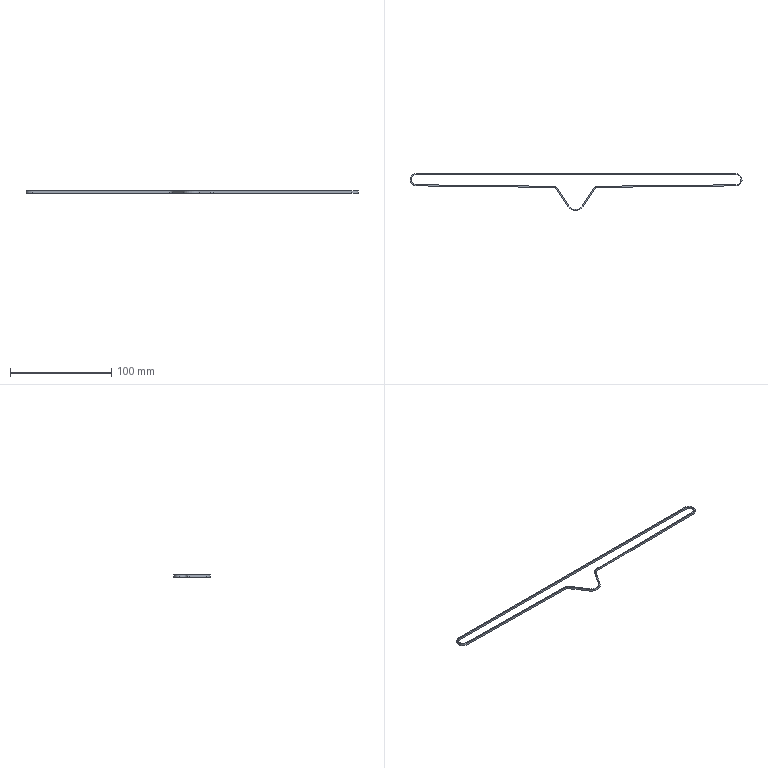Part | NX | features BREP 1 | 1 solid | 24 faces | box 328.22 x 36.55 x 2 mm | volume 1530 mm3 | plane 12 | cylinder 12 | commonest cylinder face diameters 10 x5 12.22 x3 7.78 x2 15.66 x1 17.88 x1
STEP:
#1=CARTESIAN_POINT('',(-136.555,-6.5,-1.));
#2=VERTEX_POINT('',#1);
#3=CARTESIAN_POINT('',(0.05492,-5.,-1.));
#4=VERTEX_POINT('',#3);
#5=CARTESIAN_POINT('',(0.05492,-5.,-1.));
#6=DIRECTION('',(0.9999,0.01098,0.));
#7=VECTOR('',#6,1000.);
#8=LINE('',#5,#7);
#9=EDGE_CURVE('',#2,#4,#8,.T.);
#10=ORIENTED_EDGE('',*,*,#9,.F.);
#11=CARTESIAN_POINT('',(-136.555,-6.5,1.));
#12=VERTEX_POINT('',#11);
#13=CARTESIAN_POINT('',(-136.555,-6.5,1.));
#14=DIRECTION('',(0.,0.,-1.));
#15=VECTOR('',#14,1000.);
#16=LINE('',#13,#15);
#17=EDGE_CURVE('',#12,#2,#16,.T.);
#18=ORIENTED_EDGE('',*,*,#17,.F.);
#19=CARTESIAN_POINT('',(0.05492,-5.,1.));
#20=VERTEX_POINT('',#19);
#21=CARTESIAN_POINT('',(0.05492,-5.,1.));
#22=DIRECTION('',(0.9999,0.01098,0.));
#23=VECTOR('',#22,1000.);
#24=LINE('',#21,#23);
#25=EDGE_CURVE('',#12,#20,#24,.T.);
#26=ORIENTED_EDGE('',*,*,#25,.T.);
#27=CARTESIAN_POINT('',(0.05492,-5.,1.));
#28=DIRECTION('',(0.,0.,-1.));
#29=VECTOR('',#28,1000.);
#30=LINE('',#27,#29);
#31=EDGE_CURVE('',#20,#4,#30,.T.);
#32=ORIENTED_EDGE('',*,*,#31,.T.);
#33=EDGE_LOOP('',(#10,#18,#26,#32));
#34=FACE_BOUND('',#33,.T.);
#35=CARTESIAN_POINT('',(0.05492,-5.,1.));
#36=DIRECTION('',(-0.01098,0.9999,0.));
#37=DIRECTION('',(-0.9999,-0.01098,0.));
#38=AXIS2_PLACEMENT_3D('',#35,#36,#37);
#39=PLANE('',#38);
#40=ADVANCED_FACE('',(#34),#39,.T.);
#41=CARTESIAN_POINT('',(-140.67,-8.741,-1.));
#42=VERTEX_POINT('',#41);
#43=CARTESIAN_POINT('',(-136.5,-11.5,-1.));
#44=DIRECTION('',(0.,0.,-1.));
#45=DIRECTION('',(1.,0.,0.));
#46=AXIS2_PLACEMENT_3D('',#43,#44,#45);
#47=CIRCLE('',#46,5.);
#48=EDGE_CURVE('',#42,#2,#47,.T.);
#49=ORIENTED_EDGE('',*,*,#48,.F.);
#50=CARTESIAN_POINT('',(-140.67,-8.741,1.));
#51=VERTEX_POINT('',#50);
#52=CARTESIAN_POINT('',(-140.67,-8.741,1.));
#53=DIRECTION('',(0.,0.,-1.));
#54=VECTOR('',#53,1000.);
#55=LINE('',#52,#54);
#56=EDGE_CURVE('',#51,#42,#55,.T.);
#57=ORIENTED_EDGE('',*,*,#56,.F.);
#58=CARTESIAN_POINT('',(-136.5,-11.5,1.));
#59=DIRECTION('',(0.,0.,-1.));
#60=DIRECTION('',(1.,0.,0.));
#61=AXIS2_PLACEMENT_3D('',#58,#59,#60);
#62=CIRCLE('',#61,5.);
#63=EDGE_CURVE('',#51,#12,#62,.T.);
#64=ORIENTED_EDGE('',*,*,#63,.T.);
#65=ORIENTED_EDGE('',*,*,#17,.T.);
#66=EDGE_LOOP('',(#49,#57,#64,#65));
#67=FACE_BOUND('',#66,.T.);
#68=CARTESIAN_POINT('',(-136.5,-11.5,1.));
#69=DIRECTION('',(0.,0.,-1.));
#70=DIRECTION('',(-1.,0.,0.));
#71=AXIS2_PLACEMENT_3D('',#68,#69,#70);
#72=CYLINDRICAL_SURFACE('',#71,5.);
#73=ADVANCED_FACE('',(#67),#72,.T.);
#74=CARTESIAN_POINT('',(-151.97,-25.82,-1.));
#75=VERTEX_POINT('',#74);
#76=CARTESIAN_POINT('',(-140.67,-8.741,-1.));
#77=DIRECTION('',(0.5518,0.834,0.));
#78=VECTOR('',#77,1000.);
#79=LINE('',#76,#78);
#80=EDGE_CURVE('',#75,#42,#79,.T.);
#81=ORIENTED_EDGE('',*,*,#80,.F.);
#82=CARTESIAN_POINT('',(-151.97,-25.82,1.));
#83=VERTEX_POINT('',#82);
#84=CARTESIAN_POINT('',(-151.97,-25.82,1.));
#85=DIRECTION('',(0.,0.,-1.));
#86=VECTOR('',#85,1000.);
#87=LINE('',#84,#86);
#88=EDGE_CURVE('',#83,#75,#87,.T.);
#89=ORIENTED_EDGE('',*,*,#88,.F.);
#90=CARTESIAN_POINT('',(-140.67,-8.741,1.));
#91=DIRECTION('',(0.5518,0.834,0.));
#92=VECTOR('',#91,1000.);
#93=LINE('',#90,#92);
#94=EDGE_CURVE('',#83,#51,#93,.T.);
#95=ORIENTED_EDGE('',*,*,#94,.T.);
#96=ORIENTED_EDGE('',*,*,#56,.T.);
#97=EDGE_LOOP('',(#81,#89,#95,#96));
#98=FACE_BOUND('',#97,.T.);
#99=CARTESIAN_POINT('',(-140.67,-8.741,1.));
#100=DIRECTION('',(-0.834,0.5518,0.));
#101=DIRECTION('',(-0.5518,-0.834,0.));
#102=AXIS2_PLACEMENT_3D('',#99,#100,#101);
#103=PLANE('',#102);
#104=ADVANCED_FACE('',(#98),#103,.T.);
#105=CARTESIAN_POINT('',(-165.03,-25.82,-1.));
#106=VERTEX_POINT('',#105);
#107=CARTESIAN_POINT('',(-158.5,-21.5,-1.));
#108=DIRECTION('',(0.,0.,1.));
#109=DIRECTION('',(-1.,0.,0.));
#110=AXIS2_PLACEMENT_3D('',#107,#108,#109);
#111=CIRCLE('',#110,7.83);
#112=EDGE_CURVE('',#106,#75,#111,.T.);
#113=ORIENTED_EDGE('',*,*,#112,.F.);
#114=CARTESIAN_POINT('',(-165.03,-25.82,1.));
#115=VERTEX_POINT('',#114);
#116=CARTESIAN_POINT('',(-165.03,-25.82,1.));
#117=DIRECTION('',(0.,0.,-1.));
#118=VECTOR('',#117,1000.);
#119=LINE('',#116,#118);
#120=EDGE_CURVE('',#115,#106,#119,.T.);
#121=ORIENTED_EDGE('',*,*,#120,.F.);
#122=CARTESIAN_POINT('',(-158.5,-21.5,1.));
#123=DIRECTION('',(0.,0.,1.));
#124=DIRECTION('',(-1.,0.,0.));
#125=AXIS2_PLACEMENT_3D('',#122,#123,#124);
#126=CIRCLE('',#125,7.83);
#127=EDGE_CURVE('',#115,#83,#126,.T.);
#128=ORIENTED_EDGE('',*,*,#127,.T.);
#129=ORIENTED_EDGE('',*,*,#88,.T.);
#130=EDGE_LOOP('',(#113,#121,#128,#129));
#131=FACE_BOUND('',#130,.T.);
#132=CARTESIAN_POINT('',(-158.5,-21.5,1.));
#133=DIRECTION('',(0.,0.,-1.));
#134=DIRECTION('',(-1.,0.,0.));
#135=AXIS2_PLACEMENT_3D('',#132,#133,#134);
#136=CYLINDRICAL_SURFACE('',#135,7.83);
#137=ADVANCED_FACE('',(#131),#136,.F.);
#138=CARTESIAN_POINT('',(-176.33,-8.741,-1.));
#139=VERTEX_POINT('',#138);
#140=CARTESIAN_POINT('',(-165.03,-25.82,-1.));
#141=DIRECTION('',(0.5518,-0.834,0.));
#142=VECTOR('',#141,1000.);
#143=LINE('',#140,#142);
#144=EDGE_CURVE('',#139,#106,#143,.T.);
#145=ORIENTED_EDGE('',*,*,#144,.F.);
#146=CARTESIAN_POINT('',(-176.33,-8.741,1.));
#147=VERTEX_POINT('',#146);
#148=CARTESIAN_POINT('',(-176.33,-8.741,1.));
#149=DIRECTION('',(0.,0.,-1.));
#150=VECTOR('',#149,1000.);
#151=LINE('',#148,#150);
#152=EDGE_CURVE('',#147,#139,#151,.T.);
#153=ORIENTED_EDGE('',*,*,#152,.F.);
#154=CARTESIAN_POINT('',(-165.03,-25.82,1.));
#155=DIRECTION('',(0.5518,-0.834,0.));
#156=VECTOR('',#155,1000.);
#157=LINE('',#154,#156);
#158=EDGE_CURVE('',#147,#115,#157,.T.);
#159=ORIENTED_EDGE('',*,*,#158,.T.);
#160=ORIENTED_EDGE('',*,*,#120,.T.);
#161=EDGE_LOOP('',(#145,#153,#159,#160));
#162=FACE_BOUND('',#161,.T.);
#163=CARTESIAN_POINT('',(-165.03,-25.82,1.));
#164=DIRECTION('',(0.834,0.5518,0.));
#165=DIRECTION('',(-0.5518,0.834,0.));
#166=AXIS2_PLACEMENT_3D('',#163,#164,#165);
#167=PLANE('',#166);
#168=ADVANCED_FACE('',(#162),#167,.T.);
#169=CARTESIAN_POINT('',(-180.445,-6.5,-1.));
#170=VERTEX_POINT('',#169);
#171=CARTESIAN_POINT('',(-180.5,-11.5,-1.));
#172=DIRECTION('',(0.,0.,-1.));
#173=DIRECTION('',(1.,0.,0.));
#174=AXIS2_PLACEMENT_3D('',#171,#172,#173);
#175=CIRCLE('',#174,5.);
#176=EDGE_CURVE('',#170,#139,#175,.T.);
#177=ORIENTED_EDGE('',*,*,#176,.F.);
#178=CARTESIAN_POINT('',(-180.445,-6.5,1.));
#179=VERTEX_POINT('',#178);
#180=CARTESIAN_POINT('',(-180.445,-6.5,1.));
#181=DIRECTION('',(0.,0.,-1.));
#182=VECTOR('',#181,1000.);
#183=LINE('',#180,#182);
#184=EDGE_CURVE('',#179,#170,#183,.T.);
#185=ORIENTED_EDGE('',*,*,#184,.F.);
#186=CARTESIAN_POINT('',(-180.5,-11.5,1.));
#187=DIRECTION('',(0.,0.,-1.));
#188=DIRECTION('',(1.,0.,0.));
#189=AXIS2_PLACEMENT_3D('',#186,#187,#188);
#190=CIRCLE('',#189,5.);
#191=EDGE_CURVE('',#179,#147,#190,.T.);
#192=ORIENTED_EDGE('',*,*,#191,.T.);
#193=ORIENTED_EDGE('',*,*,#152,.T.);
#194=EDGE_LOOP('',(#177,#185,#192,#193));
#195=FACE_BOUND('',#194,.T.);
#196=CARTESIAN_POINT('',(-180.5,-11.5,1.));
#197=DIRECTION('',(0.,0.,-1.));
#198=DIRECTION('',(-1.,0.,0.));
#199=AXIS2_PLACEMENT_3D('',#196,#197,#198);
#200=CYLINDRICAL_SURFACE('',#199,5.);
#201=ADVANCED_FACE('',(#195),#200,.T.);
#202=CARTESIAN_POINT('',(-316.055,-5.,-1.));
#203=VERTEX_POINT('',#202);
#204=CARTESIAN_POINT('',(-180.445,-6.5,-1.));
#205=DIRECTION('',(0.9999,-0.01106,0.));
#206=VECTOR('',#205,1000.);
#207=LINE('',#204,#206);
#208=EDGE_CURVE('',#203,#170,#207,.T.);
#209=ORIENTED_EDGE('',*,*,#208,.F.);
#210=CARTESIAN_POINT('',(-316.055,-5.,1.));
#211=VERTEX_POINT('',#210);
#212=CARTESIAN_POINT('',(-316.055,-5.,1.));
#213=DIRECTION('',(0.,0.,-1.));
#214=VECTOR('',#213,1000.);
#215=LINE('',#212,#214);
#216=EDGE_CURVE('',#211,#203,#215,.T.);
#217=ORIENTED_EDGE('',*,*,#216,.F.);
#218=CARTESIAN_POINT('',(-180.445,-6.5,1.));
#219=DIRECTION('',(0.9999,-0.01106,0.));
#220=VECTOR('',#219,1000.);
#221=LINE('',#218,#220);
#222=EDGE_CURVE('',#211,#179,#221,.T.);
#223=ORIENTED_EDGE('',*,*,#222,.T.);
#224=ORIENTED_EDGE('',*,*,#184,.T.);
#225=EDGE_LOOP('',(#209,#217,#223,#224));
#226=FACE_BOUND('',#225,.T.);
#227=CARTESIAN_POINT('',(-180.445,-6.5,1.));
#228=DIRECTION('',(0.01106,0.9999,0.));
#229=DIRECTION('',(-0.9999,0.01106,0.));
#230=AXIS2_PLACEMENT_3D('',#227,#228,#229);
#231=PLANE('',#230);
#232=ADVANCED_FACE('',(#226),#231,.T.);
#233=CARTESIAN_POINT('',(-321.,0.,1.));
#234=VERTEX_POINT('',#233);
#235=CARTESIAN_POINT('',(-321.,0.,-1.));
#236=VERTEX_POINT('',#235);
#237=CARTESIAN_POINT('',(-321.,0.,1.));
#238=DIRECTION('',(0.,0.,-1.));
#239=VECTOR('',#238,1000.);
#240=LINE('',#237,#239);
#241=EDGE_CURVE('',#234,#236,#240,.T.);
#242=ORIENTED_EDGE('',*,*,#241,.F.);
#243=CARTESIAN_POINT('',(-316.,0.,1.));
#244=DIRECTION('',(0.,0.,1.));
#245=DIRECTION('',(-1.,0.,0.));
#246=AXIS2_PLACEMENT_3D('',#243,#244,#245);
#247=CIRCLE('',#246,5.);
#248=EDGE_CURVE('',#234,#211,#247,.T.);
#249=ORIENTED_EDGE('',*,*,#248,.T.);
#250=ORIENTED_EDGE('',*,*,#216,.T.);
#251=CARTESIAN_POINT('',(-316.,0.,-1.));
#252=DIRECTION('',(0.,0.,1.));
#253=DIRECTION('',(-1.,0.,0.));
#254=AXIS2_PLACEMENT_3D('',#251,#252,#253);
#255=CIRCLE('',#254,5.);
#256=EDGE_CURVE('',#236,#203,#255,.T.);
#257=ORIENTED_EDGE('',*,*,#256,.F.);
#258=EDGE_LOOP('',(#242,#249,#250,#257));
#259=FACE_BOUND('',#258,.T.);
#260=CARTESIAN_POINT('',(-316.,0.,1.));
#261=DIRECTION('',(0.,0.,-1.));
#262=DIRECTION('',(-1.,0.,0.));
#263=AXIS2_PLACEMENT_3D('',#260,#261,#262);
#264=CYLINDRICAL_SURFACE('',#263,5.);
#265=ADVANCED_FACE('',(#259),#264,.F.);
#266=CARTESIAN_POINT('',(0.,5.,-1.));
#267=VERTEX_POINT('',#266);
#268=CARTESIAN_POINT('',(-316.,5.,-1.));
#269=VERTEX_POINT('',#268);
#270=CARTESIAN_POINT('',(-316.,5.,-1.));
#271=DIRECTION('',(-1.,0.,0.));
#272=VECTOR('',#271,1000.);
#273=LINE('',#270,#272);
#274=EDGE_CURVE('',#267,#269,#273,.T.);
#275=ORIENTED_EDGE('',*,*,#274,.F.);
#276=CARTESIAN_POINT('',(0.,5.,1.));
#277=VERTEX_POINT('',#276);
#278=CARTESIAN_POINT('',(0.,5.,1.));
#279=DIRECTION('',(0.,0.,-1.));
#280=VECTOR('',#279,1000.);
#281=LINE('',#278,#280);
#282=EDGE_CURVE('',#277,#267,#281,.T.);
#283=ORIENTED_EDGE('',*,*,#282,.F.);
#284=CARTESIAN_POINT('',(-316.,5.,1.));
#285=VERTEX_POINT('',#284);
#286=CARTESIAN_POINT('',(-316.,5.,1.));
#287=DIRECTION('',(-1.,0.,0.));
#288=VECTOR('',#287,1000.);
#289=LINE('',#286,#288);
#290=EDGE_CURVE('',#277,#285,#289,.T.);
#291=ORIENTED_EDGE('',*,*,#290,.T.);
#292=CARTESIAN_POINT('',(-316.,5.,1.));
#293=DIRECTION('',(0.,0.,-1.));
#294=VECTOR('',#293,1000.);
#295=LINE('',#292,#294);
#296=EDGE_CURVE('',#285,#269,#295,.T.);
#297=ORIENTED_EDGE('',*,*,#296,.T.);
#298=EDGE_LOOP('',(#275,#283,#291,#297));
#299=FACE_BOUND('',#298,.T.);
#300=CARTESIAN_POINT('',(-316.,5.,1.));
#301=DIRECTION('',(0.,-1.,0.));
#302=DIRECTION('',(1.,0.,0.));
#303=AXIS2_PLACEMENT_3D('',#300,#301,#302);
#304=PLANE('',#303);
#305=ADVANCED_FACE('',(#299),#304,.T.);
#306=CARTESIAN_POINT('',(0.,0.,-1.));
#307=DIRECTION('',(0.,0.,1.));
#308=DIRECTION('',(-1.,0.,0.));
#309=AXIS2_PLACEMENT_3D('',#306,#307,#308);
#310=CIRCLE('',#309,5.);
#311=EDGE_CURVE('',#4,#267,#310,.T.);
#312=ORIENTED_EDGE('',*,*,#311,.F.);
#313=ORIENTED_EDGE('',*,*,#31,.F.);
#314=CARTESIAN_POINT('',(0.,0.,1.));
#315=DIRECTION('',(0.,0.,1.));
#316=DIRECTION('',(-1.,0.,0.));
#317=AXIS2_PLACEMENT_3D('',#314,#315,#316);
#318=CIRCLE('',#317,5.);
#319=EDGE_CURVE('',#20,#277,#318,.T.);
#320=ORIENTED_EDGE('',*,*,#319,.T.);
#321=ORIENTED_EDGE('',*,*,#282,.T.);
#322=EDGE_LOOP('',(#312,#313,#320,#321));
#323=FACE_BOUND('',#322,.T.);
#324=CARTESIAN_POINT('',(0.,0.,1.));
#325=DIRECTION('',(0.,0.,-1.));
#326=DIRECTION('',(-1.,0.,0.));
#327=AXIS2_PLACEMENT_3D('',#324,#325,#326);
#328=CYLINDRICAL_SURFACE('',#327,5.);
#329=ADVANCED_FACE('',(#323),#328,.F.);
#330=CARTESIAN_POINT('',(-136.543,-7.61,-1.));
#331=VERTEX_POINT('',#330);
#332=CARTESIAN_POINT('',(0.06711,-6.11,-1.));
#333=VERTEX_POINT('',#332);
#334=CARTESIAN_POINT('',(0.06711,-6.11,-1.));
#335=DIRECTION('',(0.9999,0.01098,0.));
#336=VECTOR('',#335,1000.);
#337=LINE('',#334,#336);
#338=EDGE_CURVE('',#331,#333,#337,.T.);
#339=ORIENTED_EDGE('',*,*,#338,.T.);
#340=CARTESIAN_POINT('',(0.06711,-6.11,1.));
#341=VERTEX_POINT('',#340);
#342=CARTESIAN_POINT('',(0.06711,-6.11,1.));
#343=DIRECTION('',(0.,0.,-1.));
#344=VECTOR('',#343,1000.);
#345=LINE('',#342,#344);
#346=EDGE_CURVE('',#341,#333,#345,.T.);
#347=ORIENTED_EDGE('',*,*,#346,.F.);
#348=CARTESIAN_POINT('',(-136.543,-7.61,1.));
#349=VERTEX_POINT('',#348);
#350=CARTESIAN_POINT('',(0.06711,-6.11,1.));
#351=DIRECTION('',(0.9999,0.01098,0.));
#352=VECTOR('',#351,1000.);
#353=LINE('',#350,#352);
#354=EDGE_CURVE('',#349,#341,#353,.T.);
#355=ORIENTED_EDGE('',*,*,#354,.F.);
#356=CARTESIAN_POINT('',(-136.543,-7.61,1.));
#357=DIRECTION('',(0.,0.,-1.));
#358=VECTOR('',#357,1000.);
#359=LINE('',#356,#358);
#360=EDGE_CURVE('',#349,#331,#359,.T.);
#361=ORIENTED_EDGE('',*,*,#360,.T.);
#362=EDGE_LOOP('',(#339,#347,#355,#361));
#363=FACE_BOUND('',#362,.T.);
#364=CARTESIAN_POINT('',(0.06711,-6.11,1.));
#365=DIRECTION('',(-0.01098,0.9999,0.));
#366=DIRECTION('',(-0.9999,-0.01098,0.));
#367=AXIS2_PLACEMENT_3D('',#364,#365,#366);
#368=PLANE('',#367);
#369=ADVANCED_FACE('',(#363),#368,.F.);
#370=CARTESIAN_POINT('',(-139.744,-9.354,-1.));
#371=VERTEX_POINT('',#370);
#372=CARTESIAN_POINT('',(-136.5,-11.5,-1.));
#373=DIRECTION('',(0.,0.,-1.));
#374=DIRECTION('',(-1.,0.,0.));
#375=AXIS2_PLACEMENT_3D('',#372,#373,#374);
#376=CIRCLE('',#375,3.89);
#377=EDGE_CURVE('',#371,#331,#376,.T.);
#378=ORIENTED_EDGE('',*,*,#377,.T.);
#379=ORIENTED_EDGE('',*,*,#360,.F.);
#380=CARTESIAN_POINT('',(-139.744,-9.354,1.));
#381=VERTEX_POINT('',#380);
#382=CARTESIAN_POINT('',(-136.5,-11.5,1.));
#383=DIRECTION('',(0.,0.,-1.));
#384=DIRECTION('',(-1.,0.,0.));
#385=AXIS2_PLACEMENT_3D('',#382,#383,#384);
#386=CIRCLE('',#385,3.89);
#387=EDGE_CURVE('',#381,#349,#386,.T.);
#388=ORIENTED_EDGE('',*,*,#387,.F.);
#389=CARTESIAN_POINT('',(-139.744,-9.354,1.));
#390=DIRECTION('',(0.,0.,-1.));
#391=VECTOR('',#390,1000.);
#392=LINE('',#389,#391);
#393=EDGE_CURVE('',#381,#371,#392,.T.);
#394=ORIENTED_EDGE('',*,*,#393,.T.);
#395=EDGE_LOOP('',(#378,#379,#388,#394));
#396=FACE_BOUND('',#395,.T.);
#397=CARTESIAN_POINT('',(-136.5,-11.5,1.));
#398=DIRECTION('',(0.,0.,-1.));
#399=DIRECTION('',(-1.,0.,0.));
#400=AXIS2_PLACEMENT_3D('',#397,#398,#399);
#401=CYLINDRICAL_SURFACE('',#400,3.89);
#402=ADVANCED_FACE('',(#396),#401,.F.);
#403=CARTESIAN_POINT('',(-151.044,-26.433,-1.));
#404=VERTEX_POINT('',#403);
#405=CARTESIAN_POINT('',(-92.893,61.459,-1.));
#406=DIRECTION('',(0.5518,0.834,0.));
#407=VECTOR('',#406,1000.);
#408=LINE('',#405,#407);
#409=EDGE_CURVE('',#404,#371,#408,.T.);
#410=ORIENTED_EDGE('',*,*,#409,.T.);
#411=ORIENTED_EDGE('',*,*,#393,.F.);
#412=CARTESIAN_POINT('',(-151.044,-26.433,1.));
#413=VERTEX_POINT('',#412);
#414=CARTESIAN_POINT('',(-92.893,61.459,1.));
#415=DIRECTION('',(0.5518,0.834,0.));
#416=VECTOR('',#415,1000.);
#417=LINE('',#414,#416);
#418=EDGE_CURVE('',#413,#381,#417,.T.);
#419=ORIENTED_EDGE('',*,*,#418,.F.);
#420=CARTESIAN_POINT('',(-151.044,-26.433,1.));
#421=DIRECTION('',(0.,0.,-1.));
#422=VECTOR('',#421,1000.);
#423=LINE('',#420,#422);
#424=EDGE_CURVE('',#413,#404,#423,.T.);
#425=ORIENTED_EDGE('',*,*,#424,.T.);
#426=EDGE_LOOP('',(#410,#411,#419,#425));
#427=FACE_BOUND('',#426,.T.);
#428=CARTESIAN_POINT('',(-92.893,61.459,1.));
#429=DIRECTION('',(-0.834,0.5518,0.));
#430=DIRECTION('',(-0.5518,-0.834,0.));
#431=AXIS2_PLACEMENT_3D('',#428,#429,#430);
#432=PLANE('',#431);
#433=ADVANCED_FACE('',(#427),#432,.F.);
#434=CARTESIAN_POINT('',(-165.956,-26.433,-1.));
#435=VERTEX_POINT('',#434);
#436=CARTESIAN_POINT('',(-158.5,-21.5,-1.));
#437=DIRECTION('',(0.,0.,1.));
#438=DIRECTION('',(-1.,0.,0.));
#439=AXIS2_PLACEMENT_3D('',#436,#437,#438);
#440=CIRCLE('',#439,8.94);
#441=EDGE_CURVE('',#435,#404,#440,.T.);
#442=ORIENTED_EDGE('',*,*,#441,.T.);
#443=ORIENTED_EDGE('',*,*,#424,.F.);
#444=CARTESIAN_POINT('',(-165.956,-26.433,1.));
#445=VERTEX_POINT('',#444);
#446=CARTESIAN_POINT('',(-158.5,-21.5,1.));
#447=DIRECTION('',(0.,0.,1.));
#448=DIRECTION('',(-1.,0.,0.));
#449=AXIS2_PLACEMENT_3D('',#446,#447,#448);
#450=CIRCLE('',#449,8.94);
#451=EDGE_CURVE('',#445,#413,#450,.T.);
#452=ORIENTED_EDGE('',*,*,#451,.F.);
#453=CARTESIAN_POINT('',(-165.956,-26.433,1.));
#454=DIRECTION('',(0.,0.,-1.));
#455=VECTOR('',#454,1000.);
#456=LINE('',#453,#455);
#457=EDGE_CURVE('',#445,#435,#456,.T.);
#458=ORIENTED_EDGE('',*,*,#457,.T.);
#459=EDGE_LOOP('',(#442,#443,#452,#458));
#460=FACE_BOUND('',#459,.T.);
#461=CARTESIAN_POINT('',(-158.5,-21.5,1.));
#462=DIRECTION('',(0.,0.,-1.));
#463=DIRECTION('',(-1.,0.,0.));
#464=AXIS2_PLACEMENT_3D('',#461,#462,#463);
#465=CYLINDRICAL_SURFACE('',#464,8.94);
#466=ADVANCED_FACE('',(#460),#465,.T.);
#467=CARTESIAN_POINT('',(-177.256,-9.354,-1.));
#468=VERTEX_POINT('',#467);
#469=CARTESIAN_POINT('',(-127.593,-84.417,-1.));
#470=DIRECTION('',(0.5518,-0.834,0.));
#471=VECTOR('',#470,1000.);
#472=LINE('',#469,#471);
#473=EDGE_CURVE('',#468,#435,#472,.T.);
#474=ORIENTED_EDGE('',*,*,#473,.T.);
#475=ORIENTED_EDGE('',*,*,#457,.F.);
#476=CARTESIAN_POINT('',(-177.256,-9.354,1.));
#477=VERTEX_POINT('',#476);
#478=CARTESIAN_POINT('',(-127.593,-84.417,1.));
#479=DIRECTION('',(0.5518,-0.834,0.));
#480=VECTOR('',#479,1000.);
#481=LINE('',#478,#480);
#482=EDGE_CURVE('',#477,#445,#481,.T.);
#483=ORIENTED_EDGE('',*,*,#482,.F.);
#484=CARTESIAN_POINT('',(-177.256,-9.354,1.));
#485=DIRECTION('',(0.,0.,-1.));
#486=VECTOR('',#485,1000.);
#487=LINE('',#484,#486);
#488=EDGE_CURVE('',#477,#468,#487,.T.);
#489=ORIENTED_EDGE('',*,*,#488,.T.);
#490=EDGE_LOOP('',(#474,#475,#483,#489));
#491=FACE_BOUND('',#490,.T.);
#492=CARTESIAN_POINT('',(-127.593,-84.417,1.));
#493=DIRECTION('',(0.834,0.5518,0.));
#494=DIRECTION('',(-0.5518,0.834,0.));
#495=AXIS2_PLACEMENT_3D('',#492,#493,#494);
#496=PLANE('',#495);
#497=ADVANCED_FACE('',(#491),#496,.F.);
#498=CARTESIAN_POINT('',(-180.457,-7.61,-1.));
#499=VERTEX_POINT('',#498);
#500=CARTESIAN_POINT('',(-180.5,-11.5,-1.));
#501=DIRECTION('',(0.,0.,-1.));
#502=DIRECTION('',(-1.,0.,0.));
#503=AXIS2_PLACEMENT_3D('',#500,#501,#502);
#504=CIRCLE('',#503,3.89);
#505=EDGE_CURVE('',#499,#468,#504,.T.);
#506=ORIENTED_EDGE('',*,*,#505,.T.);
#507=ORIENTED_EDGE('',*,*,#488,.F.);
#508=CARTESIAN_POINT('',(-180.457,-7.61,1.));
#509=VERTEX_POINT('',#508);
#510=CARTESIAN_POINT('',(-180.5,-11.5,1.));
#511=DIRECTION('',(0.,0.,-1.));
#512=DIRECTION('',(-1.,0.,0.));
#513=AXIS2_PLACEMENT_3D('',#510,#511,#512);
#514=CIRCLE('',#513,3.89);
#515=EDGE_CURVE('',#509,#477,#514,.T.);
#516=ORIENTED_EDGE('',*,*,#515,.F.);
#517=CARTESIAN_POINT('',(-180.457,-7.61,1.));
#518=DIRECTION('',(0.,0.,-1.));
#519=VECTOR('',#518,1000.);
#520=LINE('',#517,#519);
#521=EDGE_CURVE('',#509,#499,#520,.T.);
#522=ORIENTED_EDGE('',*,*,#521,.T.);
#523=EDGE_LOOP('',(#506,#507,#516,#522));
#524=FACE_BOUND('',#523,.T.);
#525=CARTESIAN_POINT('',(-180.5,-11.5,1.));
#526=DIRECTION('',(0.,0.,-1.));
#527=DIRECTION('',(-1.,0.,0.));
#528=AXIS2_PLACEMENT_3D('',#525,#526,#527);
#529=CYLINDRICAL_SURFACE('',#528,3.89);
#530=ADVANCED_FACE('',(#524),#529,.F.);
#531=CARTESIAN_POINT('',(-316.068,-6.11,-1.));
#532=VERTEX_POINT('',#531);
#533=CARTESIAN_POINT('',(-0.1063,-9.606,-1.));
#534=DIRECTION('',(0.9999,-0.01106,0.));
#535=VECTOR('',#534,1000.);
#536=LINE('',#533,#535);
#537=EDGE_CURVE('',#532,#499,#536,.T.);
#538=ORIENTED_EDGE('',*,*,#537,.T.);
#539=ORIENTED_EDGE('',*,*,#521,.F.);
#540=CARTESIAN_POINT('',(-316.068,-6.11,1.));
#541=VERTEX_POINT('',#540);
#542=CARTESIAN_POINT('',(-0.1063,-9.606,1.));
#543=DIRECTION('',(0.9999,-0.01106,0.));
#544=VECTOR('',#543,1000.);
#545=LINE('',#542,#544);
#546=EDGE_CURVE('',#541,#509,#545,.T.);
#547=ORIENTED_EDGE('',*,*,#546,.F.);
#548=CARTESIAN_POINT('',(-316.068,-6.11,1.));
#549=DIRECTION('',(0.,0.,-1.));
#550=VECTOR('',#549,1000.);
#551=LINE('',#548,#550);
#552=EDGE_CURVE('',#541,#532,#551,.T.);
#553=ORIENTED_EDGE('',*,*,#552,.T.);
#554=EDGE_LOOP('',(#538,#539,#547,#553));
#555=FACE_BOUND('',#554,.T.);
#556=CARTESIAN_POINT('',(-0.1063,-9.606,1.));
#557=DIRECTION('',(0.01106,0.9999,0.));
#558=DIRECTION('',(-0.9999,0.01106,0.));
#559=AXIS2_PLACEMENT_3D('',#556,#557,#558);
#560=PLANE('',#559);
#561=ADVANCED_FACE('',(#555),#560,.F.);
#562=CARTESIAN_POINT('',(-322.11,0.,1.));
#563=VERTEX_POINT('',#562);
#564=CARTESIAN_POINT('',(-322.11,0.,-1.));
#565=VERTEX_POINT('',#564);
#566=CARTESIAN_POINT('',(-322.11,0.,1.));
#567=DIRECTION('',(0.,0.,-1.));
#568=VECTOR('',#567,1000.);
#569=LINE('',#566,#568);
#570=EDGE_CURVE('',#563,#565,#569,.T.);
#571=ORIENTED_EDGE('',*,*,#570,.F.);
#572=CARTESIAN_POINT('',(-316.,6.11,1.));
#573=VERTEX_POINT('',#572);
#574=CARTESIAN_POINT('',(-316.,0.,1.));
#575=DIRECTION('',(0.,0.,1.));
#576=DIRECTION('',(-1.,0.,0.));
#577=AXIS2_PLACEMENT_3D('',#574,#575,#576);
#578=CIRCLE('',#577,6.11);
#579=EDGE_CURVE('',#573,#563,#578,.T.);
#580=ORIENTED_EDGE('',*,*,#579,.F.);
#581=CARTESIAN_POINT('',(-316.,6.11,-1.));
#582=VERTEX_POINT('',#581);
#583=CARTESIAN_POINT('',(-316.,6.11,1.));
#584=DIRECTION('',(0.,0.,-1.));
#585=VECTOR('',#584,1000.);
#586=LINE('',#583,#585);
#587=EDGE_CURVE('',#573,#582,#586,.T.);
#588=ORIENTED_EDGE('',*,*,#587,.T.);
#589=CARTESIAN_POINT('',(-316.,0.,-1.));
#590=DIRECTION('',(0.,0.,1.));
#591=DIRECTION('',(-1.,0.,0.));
#592=AXIS2_PLACEMENT_3D('',#589,#590,#591);
#593=CIRCLE('',#592,6.11);
#594=EDGE_CURVE('',#582,#565,#593,.T.);
#595=ORIENTED_EDGE('',*,*,#594,.T.);
#596=EDGE_LOOP('',(#571,#580,#588,#595));
#597=FACE_BOUND('',#596,.T.);
#598=CARTESIAN_POINT('',(-316.,0.,1.));
#599=DIRECTION('',(0.,0.,-1.));
#600=DIRECTION('',(-1.,0.,0.));
#601=AXIS2_PLACEMENT_3D('',#598,#599,#600);
#602=CYLINDRICAL_SURFACE('',#601,6.11);
#603=ADVANCED_FACE('',(#597),#602,.T.);
#604=CARTESIAN_POINT('',(0.,6.11,-1.));
#605=VERTEX_POINT('',#604);
#606=CARTESIAN_POINT('',(0.,6.11,-1.));
#607=DIRECTION('',(-1.,0.,0.));
#608=VECTOR('',#607,1000.);
#609=LINE('',#606,#608);
#610=EDGE_CURVE('',#605,#582,#609,.T.);
#611=ORIENTED_EDGE('',*,*,#610,.T.);
#612=ORIENTED_EDGE('',*,*,#587,.F.);
#613=CARTESIAN_POINT('',(0.,6.11,1.));
#614=VERTEX_POINT('',#613);
#615=CARTESIAN_POINT('',(0.,6.11,1.));
#616=DIRECTION('',(-1.,0.,0.));
#617=VECTOR('',#616,1000.);
#618=LINE('',#615,#617);
#619=EDGE_CURVE('',#614,#573,#618,.T.);
#620=ORIENTED_EDGE('',*,*,#619,.F.);
#621=CARTESIAN_POINT('',(0.,6.11,1.));
#622=DIRECTION('',(0.,0.,-1.));
#623=VECTOR('',#622,1000.);
#624=LINE('',#621,#623);
#625=EDGE_CURVE('',#614,#605,#624,.T.);
#626=ORIENTED_EDGE('',*,*,#625,.T.);
#627=EDGE_LOOP('',(#611,#612,#620,#626));
#628=FACE_BOUND('',#627,.T.);
#629=CARTESIAN_POINT('',(0.,6.11,1.));
#630=DIRECTION('',(0.,-1.,0.));
#631=DIRECTION('',(1.,0.,0.));
#632=AXIS2_PLACEMENT_3D('',#629,#630,#631);
#633=PLANE('',#632);
#634=ADVANCED_FACE('',(#628),#633,.F.);
#635=CARTESIAN_POINT('',(0.,0.,-1.));
#636=DIRECTION('',(0.,0.,1.));
#637=DIRECTION('',(-1.,0.,0.));
#638=AXIS2_PLACEMENT_3D('',#635,#636,#637);
#639=CIRCLE('',#638,6.11);
#640=EDGE_CURVE('',#333,#605,#639,.T.);
#641=ORIENTED_EDGE('',*,*,#640,.T.);
#642=ORIENTED_EDGE('',*,*,#625,.F.);
#643=CARTESIAN_POINT('',(0.,0.,1.));
#644=DIRECTION('',(0.,0.,1.));
#645=DIRECTION('',(-1.,0.,0.));
#646=AXIS2_PLACEMENT_3D('',#643,#644,#645);
#647=CIRCLE('',#646,6.11);
#648=EDGE_CURVE('',#341,#614,#647,.T.);
#649=ORIENTED_EDGE('',*,*,#648,.F.);
#650=ORIENTED_EDGE('',*,*,#346,.T.);
#651=EDGE_LOOP('',(#641,#642,#649,#650));
#652=FACE_BOUND('',#651,.T.);
#653=CARTESIAN_POINT('',(0.,0.,1.));
#654=DIRECTION('',(0.,0.,-1.));
#655=DIRECTION('',(-1.,0.,0.));
#656=AXIS2_PLACEMENT_3D('',#653,#654,#655);
#657=CYLINDRICAL_SURFACE('',#656,6.11);
#658=ADVANCED_FACE('',(#652),#657,.T.);
#659=ORIENTED_EDGE('',*,*,#9,.T.);
#660=ORIENTED_EDGE('',*,*,#311,.T.);
#661=ORIENTED_EDGE('',*,*,#274,.T.);
#662=CARTESIAN_POINT('',(-316.,0.,-1.));
#663=DIRECTION('',(0.,0.,1.));
#664=DIRECTION('',(-1.,0.,0.));
#665=AXIS2_PLACEMENT_3D('',#662,#663,#664);
#666=CIRCLE('',#665,5.);
#667=EDGE_CURVE('',#269,#236,#666,.T.);
#668=ORIENTED_EDGE('',*,*,#667,.T.);
#669=ORIENTED_EDGE('',*,*,#256,.T.);
#670=ORIENTED_EDGE('',*,*,#208,.T.);
#671=ORIENTED_EDGE('',*,*,#176,.T.);
#672=ORIENTED_EDGE('',*,*,#144,.T.);
#673=ORIENTED_EDGE('',*,*,#112,.T.);
#674=ORIENTED_EDGE('',*,*,#80,.T.);
#675=ORIENTED_EDGE('',*,*,#48,.T.);
#676=EDGE_LOOP('',(#659,#660,#661,#668,#669,#670,#671,#672,#673,#674,#675));
#677=FACE_BOUND('',#676,.T.);
#678=ORIENTED_EDGE('',*,*,#640,.F.);
#679=ORIENTED_EDGE('',*,*,#338,.F.);
#680=ORIENTED_EDGE('',*,*,#377,.F.);
#681=ORIENTED_EDGE('',*,*,#409,.F.);
#682=ORIENTED_EDGE('',*,*,#441,.F.);
#683=ORIENTED_EDGE('',*,*,#473,.F.);
#684=ORIENTED_EDGE('',*,*,#505,.F.);
#685=ORIENTED_EDGE('',*,*,#537,.F.);
#686=CARTESIAN_POINT('',(-316.,0.,-1.));
#687=DIRECTION('',(0.,0.,1.));
#688=DIRECTION('',(-1.,0.,0.));
#689=AXIS2_PLACEMENT_3D('',#686,#687,#688);
#690=CIRCLE('',#689,6.11);
#691=EDGE_CURVE('',#565,#532,#690,.T.);
#692=ORIENTED_EDGE('',*,*,#691,.F.);
#693=ORIENTED_EDGE('',*,*,#594,.F.);
#694=ORIENTED_EDGE('',*,*,#610,.F.);
#695=EDGE_LOOP('',(#678,#679,#680,#681,#682,#683,#684,#685,#692,#693,#694));
#696=FACE_BOUND('',#695,.T.);
#697=CARTESIAN_POINT('',(0.,0.,-1.));
#698=DIRECTION('',(0.,0.,-1.));
#699=DIRECTION('',(-1.,0.,0.));
#700=AXIS2_PLACEMENT_3D('',#697,#698,#699);
#701=PLANE('',#700);
#702=ADVANCED_FACE('',(#677,#696),#701,.T.);
#703=ORIENTED_EDGE('',*,*,#319,.F.);
#704=ORIENTED_EDGE('',*,*,#25,.F.);
#705=ORIENTED_EDGE('',*,*,#63,.F.);
#706=ORIENTED_EDGE('',*,*,#94,.F.);
#707=ORIENTED_EDGE('',*,*,#127,.F.);
#708=ORIENTED_EDGE('',*,*,#158,.F.);
#709=ORIENTED_EDGE('',*,*,#191,.F.);
#710=ORIENTED_EDGE('',*,*,#222,.F.);
#711=ORIENTED_EDGE('',*,*,#248,.F.);
#712=CARTESIAN_POINT('',(-316.,0.,1.));
#713=DIRECTION('',(0.,0.,1.));
#714=DIRECTION('',(-1.,0.,0.));
#715=AXIS2_PLACEMENT_3D('',#712,#713,#714);
#716=CIRCLE('',#715,5.);
#717=EDGE_CURVE('',#285,#234,#716,.T.);
#718=ORIENTED_EDGE('',*,*,#717,.F.);
#719=ORIENTED_EDGE('',*,*,#290,.F.);
#720=EDGE_LOOP('',(#703,#704,#705,#706,#707,#708,#709,#710,#711,#718,#719));
#721=FACE_BOUND('',#720,.T.);
#722=ORIENTED_EDGE('',*,*,#648,.T.);
#723=ORIENTED_EDGE('',*,*,#619,.T.);
#724=ORIENTED_EDGE('',*,*,#579,.T.);
#725=CARTESIAN_POINT('',(-316.,0.,1.));
#726=DIRECTION('',(0.,0.,1.));
#727=DIRECTION('',(-1.,0.,0.));
#728=AXIS2_PLACEMENT_3D('',#725,#726,#727);
#729=CIRCLE('',#728,6.11);
#730=EDGE_CURVE('',#563,#541,#729,.T.);
#731=ORIENTED_EDGE('',*,*,#730,.T.);
#732=ORIENTED_EDGE('',*,*,#546,.T.);
#733=ORIENTED_EDGE('',*,*,#515,.T.);
#734=ORIENTED_EDGE('',*,*,#482,.T.);
#735=ORIENTED_EDGE('',*,*,#451,.T.);
#736=ORIENTED_EDGE('',*,*,#418,.T.);
#737=ORIENTED_EDGE('',*,*,#387,.T.);
#738=ORIENTED_EDGE('',*,*,#354,.T.);
#739=EDGE_LOOP('',(#722,#723,#724,#731,#732,#733,#734,#735,#736,#737,#738));
#740=FACE_BOUND('',#739,.T.);
#741=CARTESIAN_POINT('',(0.,0.,1.));
#742=DIRECTION('',(0.,0.,-1.));
#743=DIRECTION('',(-1.,0.,0.));
#744=AXIS2_PLACEMENT_3D('',#741,#742,#743);
#745=PLANE('',#744);
#746=ADVANCED_FACE('',(#721,#740),#745,.F.);
#747=ORIENTED_EDGE('',*,*,#730,.F.);
#748=ORIENTED_EDGE('',*,*,#570,.T.);
#749=ORIENTED_EDGE('',*,*,#691,.T.);
#750=ORIENTED_EDGE('',*,*,#552,.F.);
#751=EDGE_LOOP('',(#747,#748,#749,#750));
#752=FACE_BOUND('',#751,.T.);
#753=CARTESIAN_POINT('',(-316.,0.,1.));
#754=DIRECTION('',(0.,0.,-1.));
#755=DIRECTION('',(-1.,0.,0.));
#756=AXIS2_PLACEMENT_3D('',#753,#754,#755);
#757=CYLINDRICAL_SURFACE('',#756,6.11);
#758=ADVANCED_FACE('',(#752),#757,.T.);
#759=ORIENTED_EDGE('',*,*,#717,.T.);
#760=ORIENTED_EDGE('',*,*,#241,.T.);
#761=ORIENTED_EDGE('',*,*,#667,.F.);
#762=ORIENTED_EDGE('',*,*,#296,.F.);
#763=EDGE_LOOP('',(#759,#760,#761,#762));
#764=FACE_BOUND('',#763,.T.);
#765=CARTESIAN_POINT('',(-316.,0.,1.));
#766=DIRECTION('',(0.,0.,-1.));
#767=DIRECTION('',(-1.,0.,0.));
#768=AXIS2_PLACEMENT_3D('',#765,#766,#767);
#769=CYLINDRICAL_SURFACE('',#768,5.);
#770=ADVANCED_FACE('',(#764),#769,.F.);
#771=CLOSED_SHELL('',(#40,#73,#104,#137,#168,#201,#232,#265,#305,#329,#369,#402,#433,#466,#497,#530,#561,#603,#634,#658,#702,#746,#758,#770));
#772=MANIFOLD_SOLID_BREP('',#771);
#773=(LENGTH_UNIT()NAMED_UNIT(*)SI_UNIT(.MILLI.,.METRE.));
#774=UNCERTAINTY_MEASURE_WITH_UNIT(LENGTH_MEASURE(0.00001),#773,'','');
#775=(NAMED_UNIT(*)PLANE_ANGLE_UNIT()SI_UNIT($,.RADIAN.));
#776=(NAMED_UNIT(*)SI_UNIT($,.STERADIAN.)SOLID_ANGLE_UNIT());
#777=(GEOMETRIC_REPRESENTATION_CONTEXT(3)GLOBAL_UNCERTAINTY_ASSIGNED_CONTEXT((#774))GLOBAL_UNIT_ASSIGNED_CONTEXT((#773,#775,#776))REPRESENTATION_CONTEXT('',''));
#778=ADVANCED_BREP_SHAPE_REPRESENTATION('',(#772),#777);